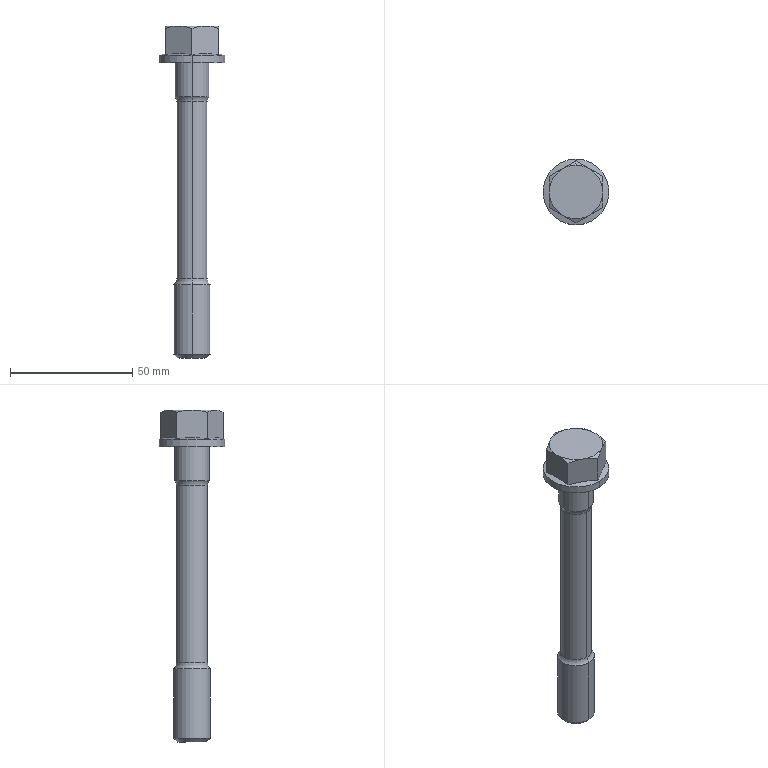Part | SolidWorks | features BaseBody 1 | 1 solid | 32 faces | box 27 x 27 x 136 mm | volume 23989 mm3 | cone 11 | plane 9 | cylinder 8 | torus 4 | commonest cylinder face diameters 12.7 x2 14 x2 15 x2 27 x2
STEP:
#1=CARTESIAN_POINT('',(-97.5,217.526,423.15));
#2=VERTEX_POINT('',#1);
#3=CARTESIAN_POINT('',(-92.,219.,423.15));
#4=VERTEX_POINT('',#3);
#5=CARTESIAN_POINT('',(-92.,208.,423.15));
#6=DIRECTION('',(0.,0.,-1.));
#7=DIRECTION('',(0.,-1.,0.));
#8=AXIS2_PLACEMENT_3D('',#5,#6,#7);
#9=CIRCLE('',#8,11.);
#10=EDGE_CURVE('',#2,#4,#9,.T.);
#11=ORIENTED_EDGE('',*,*,#10,.T.);
#12=CARTESIAN_POINT('',(-92.,220.702,422.168));
#13=VERTEX_POINT('',#12);
#14=CARTESIAN_POINT('',(-92.,216.604,424.533));
#15=DIRECTION('',(0.,0.866,-0.5));
#16=VECTOR('',#15,1000.);
#17=LINE('',#14,#16);
#18=EDGE_CURVE('',#4,#13,#17,.T.);
#19=ORIENTED_EDGE('',*,*,#18,.T.);
#20=CARTESIAN_POINT('',(-92.,220.702,422.168));
#21=CARTESIAN_POINT('',(-92.898,220.183,422.467));
#22=CARTESIAN_POINT('',(-93.804,219.66,422.714));
#23=CARTESIAN_POINT('',(-95.635,218.603,423.056));
#24=CARTESIAN_POINT('',(-96.561,218.068,423.15));
#25=CARTESIAN_POINT('',(-97.5,217.526,423.15));
#26=B_SPLINE_CURVE_WITH_KNOTS('',3,(#20,#21,#22,#23,#24,#25),.UNSPECIFIED.,.F.,.F.,(4,2,4),(0.,0.003213,0.006426),.UNSPECIFIED.);
#27=EDGE_CURVE('',#13,#2,#26,.T.);
#28=ORIENTED_EDGE('',*,*,#27,.T.);
#29=EDGE_LOOP('',(#11,#19,#28));
#30=FACE_OUTER_BOUND('',#29,.T.);
#31=CARTESIAN_POINT('',(-92.,208.,424.533));
#32=DIRECTION('',(0.,0.,-1.));
#33=DIRECTION('',(0.,1.,0.));
#34=AXIS2_PLACEMENT_3D('',#31,#32,#33);
#35=CONICAL_SURFACE('',#34,8.604,1.047);
#36=ADVANCED_FACE('',(#30),#35,.T.);
#37=CARTESIAN_POINT('',(-92.,221.5,411.15));
#38=VERTEX_POINT('',#37);
#39=CARTESIAN_POINT('',(-92.,194.5,411.15));
#40=VERTEX_POINT('',#39);
#41=CARTESIAN_POINT('',(-92.,208.,411.15));
#42=DIRECTION('',(0.,0.,-1.));
#43=DIRECTION('',(0.,1.,0.));
#44=AXIS2_PLACEMENT_3D('',#41,#42,#43);
#45=CIRCLE('',#44,13.5);
#46=EDGE_CURVE('',#38,#40,#45,.T.);
#47=ORIENTED_EDGE('',*,*,#46,.T.);
#48=CARTESIAN_POINT('',(-92.,194.5,408.15));
#49=VERTEX_POINT('',#48);
#50=CARTESIAN_POINT('',(-92.,194.5,414.767));
#51=DIRECTION('',(0.,0.,-1.));
#52=VECTOR('',#51,1000.);
#53=LINE('',#50,#52);
#54=EDGE_CURVE('',#40,#49,#53,.T.);
#55=ORIENTED_EDGE('',*,*,#54,.T.);
#56=CARTESIAN_POINT('',(-92.,221.5,408.15));
#57=VERTEX_POINT('',#56);
#58=CARTESIAN_POINT('',(-92.,208.,408.15));
#59=DIRECTION('',(0.,0.,-1.));
#60=DIRECTION('',(0.,1.,0.));
#61=AXIS2_PLACEMENT_3D('',#58,#59,#60);
#62=CIRCLE('',#61,13.5);
#63=EDGE_CURVE('',#57,#49,#62,.T.);
#64=ORIENTED_EDGE('',*,*,#63,.F.);
#65=CARTESIAN_POINT('',(-92.,221.5,414.767));
#66=DIRECTION('',(0.,0.,-1.));
#67=VECTOR('',#66,1000.);
#68=LINE('',#65,#67);
#69=EDGE_CURVE('',#38,#57,#68,.T.);
#70=ORIENTED_EDGE('',*,*,#69,.F.);
#71=EDGE_LOOP('',(#47,#55,#64,#70));
#72=FACE_OUTER_BOUND('',#71,.T.);
#73=CARTESIAN_POINT('',(-92.,208.,414.767));
#74=DIRECTION('',(0.,0.,-1.));
#75=DIRECTION('',(0.,1.,0.));
#76=AXIS2_PLACEMENT_3D('',#73,#74,#75);
#77=CYLINDRICAL_SURFACE('',#76,13.5);
#78=ADVANCED_FACE('',(#72),#77,.T.);
#79=CARTESIAN_POINT('',(-81.,201.649,411.364));
#80=VERTEX_POINT('',#79);
#81=CARTESIAN_POINT('',(-92.,195.298,411.364));
#82=VERTEX_POINT('',#81);
#83=CARTESIAN_POINT('',(-81.,201.649,411.364));
#84=CARTESIAN_POINT('',(-81.917,201.12,411.506));
#85=CARTESIAN_POINT('',(-82.833,200.591,411.621));
#86=CARTESIAN_POINT('',(-84.667,199.532,411.778));
#87=CARTESIAN_POINT('',(-86.5,198.474,411.862));
#88=CARTESIAN_POINT('',(-88.333,197.415,411.778));
#89=CARTESIAN_POINT('',(-90.167,196.357,411.621));
#90=CARTESIAN_POINT('',(-91.083,195.828,411.506));
#91=CARTESIAN_POINT('',(-92.,195.298,411.364));
#92=B_SPLINE_CURVE_WITH_KNOTS('',3,(#83,#84,#85,#86,#87,#88,#89,#90,#91),.UNSPECIFIED.,.F.,.F.,(4,2,1,2,4),(0.,0.003175,0.006351,0.009526,0.0127),.UNSPECIFIED.);
#93=EDGE_CURVE('',#80,#82,#92,.T.);
#94=ORIENTED_EDGE('',*,*,#93,.T.);
#95=CARTESIAN_POINT('',(-92.,194.5,411.15));
#96=DIRECTION('',(0.,-0.9659,-0.2588));
#97=VECTOR('',#96,1000.);
#98=LINE('',#95,#97);
#99=EDGE_CURVE('',#82,#40,#98,.T.);
#100=ORIENTED_EDGE('',*,*,#99,.T.);
#101=ORIENTED_EDGE('',*,*,#46,.F.);
#102=CARTESIAN_POINT('',(-92.,220.702,411.364));
#103=VERTEX_POINT('',#102);
#104=CARTESIAN_POINT('',(-92.,221.5,411.15));
#105=DIRECTION('',(0.,0.9659,-0.2588));
#106=VECTOR('',#105,1000.);
#107=LINE('',#104,#106);
#108=EDGE_CURVE('',#103,#38,#107,.T.);
#109=ORIENTED_EDGE('',*,*,#108,.F.);
#110=CARTESIAN_POINT('',(-81.,214.351,411.364));
#111=VERTEX_POINT('',#110);
#112=CARTESIAN_POINT('',(-92.,220.702,411.364));
#113=CARTESIAN_POINT('',(-91.083,220.172,411.506));
#114=CARTESIAN_POINT('',(-90.167,219.643,411.621));
#115=CARTESIAN_POINT('',(-88.333,218.585,411.778));
#116=CARTESIAN_POINT('',(-86.5,217.526,411.862));
#117=CARTESIAN_POINT('',(-84.667,216.468,411.778));
#118=CARTESIAN_POINT('',(-82.833,215.409,411.621));
#119=CARTESIAN_POINT('',(-81.917,214.88,411.506));
#120=CARTESIAN_POINT('',(-81.,214.351,411.364));
#121=B_SPLINE_CURVE_WITH_KNOTS('',3,(#112,#113,#114,#115,#116,#117,#118,#119,#120),.UNSPECIFIED.,.F.,.F.,(4,2,1,2,4),(0.,0.003175,0.006351,0.009526,0.0127),.UNSPECIFIED.);
#122=EDGE_CURVE('',#103,#111,#121,.T.);
#123=ORIENTED_EDGE('',*,*,#122,.T.);
#124=CARTESIAN_POINT('',(-81.,214.351,411.364));
#125=CARTESIAN_POINT('',(-81.,213.292,411.506));
#126=CARTESIAN_POINT('',(-81.,212.234,411.621));
#127=CARTESIAN_POINT('',(-81.,210.117,411.778));
#128=CARTESIAN_POINT('',(-81.,208.,411.862));
#129=CARTESIAN_POINT('',(-81.,205.883,411.778));
#130=CARTESIAN_POINT('',(-81.,203.766,411.621));
#131=CARTESIAN_POINT('',(-81.,202.708,411.506));
#132=CARTESIAN_POINT('',(-81.,201.649,411.364));
#133=B_SPLINE_CURVE_WITH_KNOTS('',3,(#124,#125,#126,#127,#128,#129,#130,#131,#132),.UNSPECIFIED.,.F.,.F.,(4,2,1,2,4),(0.,0.003175,0.006351,0.009526,0.0127),.UNSPECIFIED.);
#134=EDGE_CURVE('',#111,#80,#133,.T.);
#135=ORIENTED_EDGE('',*,*,#134,.T.);
#136=EDGE_LOOP('',(#94,#100,#101,#109,#123,#135));
#137=FACE_OUTER_BOUND('',#136,.T.);
#138=CARTESIAN_POINT('',(-92.,208.,411.15));
#139=DIRECTION('',(0.,0.,-1.));
#140=DIRECTION('',(0.,1.,0.));
#141=AXIS2_PLACEMENT_3D('',#138,#139,#140);
#142=CONICAL_SURFACE('',#141,13.5,1.309);
#143=ADVANCED_FACE('',(#137),#142,.T.);
#144=CARTESIAN_POINT('',(-92.,215.,408.15));
#145=VERTEX_POINT('',#144);
#146=CARTESIAN_POINT('',(-92.,201.,408.15));
#147=VERTEX_POINT('',#146);
#148=CARTESIAN_POINT('',(-92.,208.,408.15));
#149=DIRECTION('',(0.,0.,-1.));
#150=DIRECTION('',(0.,-1.,0.));
#151=AXIS2_PLACEMENT_3D('',#148,#149,#150);
#152=CIRCLE('',#151,7.);
#153=EDGE_CURVE('',#145,#147,#152,.T.);
#154=ORIENTED_EDGE('',*,*,#153,.T.);
#155=CARTESIAN_POINT('',(-92.,201.,394.15));
#156=VERTEX_POINT('',#155);
#157=CARTESIAN_POINT('',(-92.,201.,414.767));
#158=DIRECTION('',(0.,0.,-1.));
#159=VECTOR('',#158,1000.);
#160=LINE('',#157,#159);
#161=EDGE_CURVE('',#147,#156,#160,.T.);
#162=ORIENTED_EDGE('',*,*,#161,.T.);
#163=CARTESIAN_POINT('',(-92.,215.,394.15));
#164=VERTEX_POINT('',#163);
#165=CARTESIAN_POINT('',(-92.,208.,394.15));
#166=DIRECTION('',(0.,0.,-1.));
#167=DIRECTION('',(0.,1.,0.));
#168=AXIS2_PLACEMENT_3D('',#165,#166,#167);
#169=CIRCLE('',#168,7.);
#170=EDGE_CURVE('',#164,#156,#169,.T.);
#171=ORIENTED_EDGE('',*,*,#170,.F.);
#172=CARTESIAN_POINT('',(-92.,215.,414.767));
#173=DIRECTION('',(0.,0.,-1.));
#174=VECTOR('',#173,1000.);
#175=LINE('',#172,#174);
#176=EDGE_CURVE('',#145,#164,#175,.T.);
#177=ORIENTED_EDGE('',*,*,#176,.F.);
#178=EDGE_LOOP('',(#154,#162,#171,#177));
#179=FACE_OUTER_BOUND('',#178,.T.);
#180=CARTESIAN_POINT('',(-92.,208.,414.767));
#181=DIRECTION('',(0.,0.,-1.));
#182=DIRECTION('',(0.,1.,0.));
#183=AXIS2_PLACEMENT_3D('',#180,#181,#182);
#184=CYLINDRICAL_SURFACE('',#183,7.);
#185=ADVANCED_FACE('',(#179),#184,.T.);
#186=CARTESIAN_POINT('',(-92.,201.65,392.285));
#187=VERTEX_POINT('',#186);
#188=CARTESIAN_POINT('',(-92.,214.35,392.285));
#189=VERTEX_POINT('',#188);
#190=CARTESIAN_POINT('',(-92.,208.,392.285));
#191=DIRECTION('',(0.,0.,-1.));
#192=DIRECTION('',(0.,1.,0.));
#193=AXIS2_PLACEMENT_3D('',#190,#191,#192);
#194=CIRCLE('',#193,6.35);
#195=EDGE_CURVE('',#187,#189,#194,.T.);
#196=ORIENTED_EDGE('',*,*,#195,.F.);
#197=CARTESIAN_POINT('',(-92.,198.65,392.285));
#198=DIRECTION('',(1.,0.,0.));
#199=DIRECTION('',(0.,1.,0.));
#200=AXIS2_PLACEMENT_3D('',#197,#198,#199);
#201=CIRCLE('',#200,3.);
#202=EDGE_CURVE('',#187,#156,#201,.T.);
#203=ORIENTED_EDGE('',*,*,#202,.T.);
#204=CARTESIAN_POINT('',(-92.,208.,394.15));
#205=DIRECTION('',(0.,0.,-1.));
#206=DIRECTION('',(0.,1.,0.));
#207=AXIS2_PLACEMENT_3D('',#204,#205,#206);
#208=CIRCLE('',#207,7.);
#209=EDGE_CURVE('',#156,#164,#208,.T.);
#210=ORIENTED_EDGE('',*,*,#209,.T.);
#211=CARTESIAN_POINT('',(-92.,217.35,392.285));
#212=DIRECTION('',(-1.,0.,0.));
#213=DIRECTION('',(0.,0.,1.));
#214=AXIS2_PLACEMENT_3D('',#211,#212,#213);
#215=CIRCLE('',#214,3.);
#216=EDGE_CURVE('',#189,#164,#215,.T.);
#217=ORIENTED_EDGE('',*,*,#216,.F.);
#218=EDGE_LOOP('',(#196,#203,#210,#217));
#219=FACE_OUTER_BOUND('',#218,.T.);
#220=CARTESIAN_POINT('',(-92.,208.,392.285));
#221=DIRECTION('',(0.,0.,-1.));
#222=DIRECTION('',(0.,1.,0.));
#223=AXIS2_PLACEMENT_3D('',#220,#221,#222);
#224=TOROIDAL_SURFACE('',#223,9.35,3.);
#225=ADVANCED_FACE('',(#219),#224,.F.);
#226=CARTESIAN_POINT('',(-92.,208.,392.285));
#227=DIRECTION('',(0.,0.,-1.));
#228=DIRECTION('',(0.,1.,0.));
#229=AXIS2_PLACEMENT_3D('',#226,#227,#228);
#230=CIRCLE('',#229,6.35);
#231=EDGE_CURVE('',#189,#187,#230,.T.);
#232=ORIENTED_EDGE('',*,*,#231,.T.);
#233=CARTESIAN_POINT('',(-92.,201.65,319.512));
#234=VERTEX_POINT('',#233);
#235=CARTESIAN_POINT('',(-92.,201.65,414.767));
#236=DIRECTION('',(0.,0.,-1.));
#237=VECTOR('',#236,1000.);
#238=LINE('',#235,#237);
#239=EDGE_CURVE('',#187,#234,#238,.T.);
#240=ORIENTED_EDGE('',*,*,#239,.T.);
#241=CARTESIAN_POINT('',(-92.,214.35,319.512));
#242=VERTEX_POINT('',#241);
#243=CARTESIAN_POINT('',(-92.,208.,319.512));
#244=DIRECTION('',(0.,0.,-1.));
#245=DIRECTION('',(0.,1.,0.));
#246=AXIS2_PLACEMENT_3D('',#243,#244,#245);
#247=CIRCLE('',#246,6.35);
#248=EDGE_CURVE('',#242,#234,#247,.T.);
#249=ORIENTED_EDGE('',*,*,#248,.F.);
#250=CARTESIAN_POINT('',(-92.,214.35,414.767));
#251=DIRECTION('',(0.,0.,-1.));
#252=VECTOR('',#251,1000.);
#253=LINE('',#250,#252);
#254=EDGE_CURVE('',#189,#242,#253,.T.);
#255=ORIENTED_EDGE('',*,*,#254,.F.);
#256=EDGE_LOOP('',(#232,#240,#249,#255));
#257=FACE_OUTER_BOUND('',#256,.T.);
#258=CARTESIAN_POINT('',(-92.,208.,414.767));
#259=DIRECTION('',(0.,0.,-1.));
#260=DIRECTION('',(0.,1.,0.));
#261=AXIS2_PLACEMENT_3D('',#258,#259,#260);
#262=CYLINDRICAL_SURFACE('',#261,6.35);
#263=ADVANCED_FACE('',(#257),#262,.T.);
#264=CARTESIAN_POINT('',(-92.,200.5,317.15));
#265=VERTEX_POINT('',#264);
#266=CARTESIAN_POINT('',(-92.,215.5,317.15));
#267=VERTEX_POINT('',#266);
#268=CARTESIAN_POINT('',(-92.,208.,317.15));
#269=DIRECTION('',(0.,0.,-1.));
#270=DIRECTION('',(0.,1.,0.));
#271=AXIS2_PLACEMENT_3D('',#268,#269,#270);
#272=CIRCLE('',#271,7.5);
#273=EDGE_CURVE('',#265,#267,#272,.T.);
#274=ORIENTED_EDGE('',*,*,#273,.F.);
#275=CARTESIAN_POINT('',(-92.,198.65,319.512));
#276=DIRECTION('',(1.,0.,0.));
#277=DIRECTION('',(0.,1.,0.));
#278=AXIS2_PLACEMENT_3D('',#275,#276,#277);
#279=CIRCLE('',#278,3.);
#280=EDGE_CURVE('',#265,#234,#279,.T.);
#281=ORIENTED_EDGE('',*,*,#280,.T.);
#282=CARTESIAN_POINT('',(-92.,208.,319.512));
#283=DIRECTION('',(0.,0.,-1.));
#284=DIRECTION('',(0.,1.,0.));
#285=AXIS2_PLACEMENT_3D('',#282,#283,#284);
#286=CIRCLE('',#285,6.35);
#287=EDGE_CURVE('',#234,#242,#286,.T.);
#288=ORIENTED_EDGE('',*,*,#287,.T.);
#289=CARTESIAN_POINT('',(-92.,217.35,319.512));
#290=DIRECTION('',(-1.,0.,0.));
#291=DIRECTION('',(0.,0.,1.));
#292=AXIS2_PLACEMENT_3D('',#289,#290,#291);
#293=CIRCLE('',#292,3.);
#294=EDGE_CURVE('',#267,#242,#293,.T.);
#295=ORIENTED_EDGE('',*,*,#294,.F.);
#296=EDGE_LOOP('',(#274,#281,#288,#295));
#297=FACE_OUTER_BOUND('',#296,.T.);
#298=CARTESIAN_POINT('',(-92.,208.,319.512));
#299=DIRECTION('',(0.,0.,-1.));
#300=DIRECTION('',(0.,1.,0.));
#301=AXIS2_PLACEMENT_3D('',#298,#299,#300);
#302=TOROIDAL_SURFACE('',#301,9.35,3.);
#303=ADVANCED_FACE('',(#297),#302,.F.);
#304=CARTESIAN_POINT('',(-92.,208.,317.15));
#305=DIRECTION('',(0.,0.,-1.));
#306=DIRECTION('',(0.,1.,0.));
#307=AXIS2_PLACEMENT_3D('',#304,#305,#306);
#308=CIRCLE('',#307,7.5);
#309=EDGE_CURVE('',#267,#265,#308,.T.);
#310=ORIENTED_EDGE('',*,*,#309,.T.);
#311=CARTESIAN_POINT('',(-92.,200.5,288.65));
#312=VERTEX_POINT('',#311);
#313=CARTESIAN_POINT('',(-92.,200.5,414.767));
#314=DIRECTION('',(0.,0.,-1.));
#315=VECTOR('',#314,1000.);
#316=LINE('',#313,#315);
#317=EDGE_CURVE('',#265,#312,#316,.T.);
#318=ORIENTED_EDGE('',*,*,#317,.T.);
#319=CARTESIAN_POINT('',(-92.,215.5,288.65));
#320=VERTEX_POINT('',#319);
#321=CARTESIAN_POINT('',(-92.,208.,288.65));
#322=DIRECTION('',(0.,0.,-1.));
#323=DIRECTION('',(0.,1.,0.));
#324=AXIS2_PLACEMENT_3D('',#321,#322,#323);
#325=CIRCLE('',#324,7.5);
#326=EDGE_CURVE('',#320,#312,#325,.T.);
#327=ORIENTED_EDGE('',*,*,#326,.F.);
#328=CARTESIAN_POINT('',(-92.,215.5,414.767));
#329=DIRECTION('',(0.,0.,-1.));
#330=VECTOR('',#329,1000.);
#331=LINE('',#328,#330);
#332=EDGE_CURVE('',#267,#320,#331,.T.);
#333=ORIENTED_EDGE('',*,*,#332,.F.);
#334=EDGE_LOOP('',(#310,#318,#327,#333));
#335=FACE_OUTER_BOUND('',#334,.T.);
#336=CARTESIAN_POINT('',(-92.,208.,414.767));
#337=DIRECTION('',(0.,0.,-1.));
#338=DIRECTION('',(0.,1.,0.));
#339=AXIS2_PLACEMENT_3D('',#336,#337,#338);
#340=CYLINDRICAL_SURFACE('',#339,7.5);
#341=ADVANCED_FACE('',(#335),#340,.T.);
#342=CARTESIAN_POINT('',(-92.,214.,287.15));
#343=VERTEX_POINT('',#342);
#344=CARTESIAN_POINT('',(-92.,202.,287.15));
#345=VERTEX_POINT('',#344);
#346=CARTESIAN_POINT('',(-92.,208.,287.15));
#347=DIRECTION('',(0.,0.,-1.));
#348=DIRECTION('',(0.,1.,0.));
#349=AXIS2_PLACEMENT_3D('',#346,#347,#348);
#350=CIRCLE('',#349,6.);
#351=EDGE_CURVE('',#343,#345,#350,.T.);
#352=ORIENTED_EDGE('',*,*,#351,.F.);
#353=CARTESIAN_POINT('',(-92.,214.,287.15));
#354=DIRECTION('',(0.,0.7071,0.7071));
#355=VECTOR('',#354,1000.);
#356=LINE('',#353,#355);
#357=EDGE_CURVE('',#343,#320,#356,.T.);
#358=ORIENTED_EDGE('',*,*,#357,.T.);
#359=ORIENTED_EDGE('',*,*,#326,.T.);
#360=CARTESIAN_POINT('',(-92.,202.,287.15));
#361=DIRECTION('',(0.,-0.7071,0.7071));
#362=VECTOR('',#361,1000.);
#363=LINE('',#360,#362);
#364=EDGE_CURVE('',#345,#312,#363,.T.);
#365=ORIENTED_EDGE('',*,*,#364,.F.);
#366=EDGE_LOOP('',(#352,#358,#359,#365));
#367=FACE_OUTER_BOUND('',#366,.T.);
#368=CARTESIAN_POINT('',(-92.,208.,287.15));
#369=DIRECTION('',(0.,0.,1.));
#370=DIRECTION('',(0.,-1.,0.));
#371=AXIS2_PLACEMENT_3D('',#368,#369,#370);
#372=CONICAL_SURFACE('',#371,6.,0.7854);
#373=ADVANCED_FACE('',(#367),#372,.T.);
#374=CARTESIAN_POINT('',(-92.,208.,287.15));
#375=DIRECTION('',(0.,0.,-1.));
#376=DIRECTION('',(0.,1.,0.));
#377=AXIS2_PLACEMENT_3D('',#374,#375,#376);
#378=CIRCLE('',#377,6.);
#379=EDGE_CURVE('',#345,#343,#378,.T.);
#380=ORIENTED_EDGE('',*,*,#379,.T.);
#381=ORIENTED_EDGE('',*,*,#351,.T.);
#382=EDGE_LOOP('',(#380,#381));
#383=FACE_OUTER_BOUND('',#382,.T.);
#384=CARTESIAN_POINT('',(-92.,208.,287.15));
#385=DIRECTION('',(0.,0.,-1.));
#386=DIRECTION('',(0.,-1.,0.));
#387=AXIS2_PLACEMENT_3D('',#384,#385,#386);
#388=PLANE('',#387);
#389=ADVANCED_FACE('',(#383),#388,.T.);
#390=ORIENTED_EDGE('',*,*,#357,.F.);
#391=ORIENTED_EDGE('',*,*,#379,.F.);
#392=ORIENTED_EDGE('',*,*,#364,.T.);
#393=CARTESIAN_POINT('',(-92.,208.,288.65));
#394=DIRECTION('',(0.,0.,-1.));
#395=DIRECTION('',(0.,1.,0.));
#396=AXIS2_PLACEMENT_3D('',#393,#394,#395);
#397=CIRCLE('',#396,7.5);
#398=EDGE_CURVE('',#312,#320,#397,.T.);
#399=ORIENTED_EDGE('',*,*,#398,.T.);
#400=EDGE_LOOP('',(#390,#391,#392,#399));
#401=FACE_OUTER_BOUND('',#400,.T.);
#402=CARTESIAN_POINT('',(-92.,208.,287.15));
#403=DIRECTION('',(0.,0.,1.));
#404=DIRECTION('',(0.,-1.,0.));
#405=AXIS2_PLACEMENT_3D('',#402,#403,#404);
#406=CONICAL_SURFACE('',#405,6.,0.7854);
#407=ADVANCED_FACE('',(#401),#406,.T.);
#408=ORIENTED_EDGE('',*,*,#317,.F.);
#409=ORIENTED_EDGE('',*,*,#273,.T.);
#410=ORIENTED_EDGE('',*,*,#332,.T.);
#411=ORIENTED_EDGE('',*,*,#398,.F.);
#412=EDGE_LOOP('',(#408,#409,#410,#411));
#413=FACE_OUTER_BOUND('',#412,.T.);
#414=CARTESIAN_POINT('',(-92.,208.,414.767));
#415=DIRECTION('',(0.,0.,-1.));
#416=DIRECTION('',(0.,1.,0.));
#417=AXIS2_PLACEMENT_3D('',#414,#415,#416);
#418=CYLINDRICAL_SURFACE('',#417,7.5);
#419=ADVANCED_FACE('',(#413),#418,.T.);
#420=ORIENTED_EDGE('',*,*,#280,.F.);
#421=ORIENTED_EDGE('',*,*,#309,.F.);
#422=ORIENTED_EDGE('',*,*,#294,.T.);
#423=ORIENTED_EDGE('',*,*,#248,.T.);
#424=EDGE_LOOP('',(#420,#421,#422,#423));
#425=FACE_OUTER_BOUND('',#424,.T.);
#426=CARTESIAN_POINT('',(-92.,208.,319.512));
#427=DIRECTION('',(0.,0.,-1.));
#428=DIRECTION('',(0.,1.,0.));
#429=AXIS2_PLACEMENT_3D('',#426,#427,#428);
#430=TOROIDAL_SURFACE('',#429,9.35,3.);
#431=ADVANCED_FACE('',(#425),#430,.F.);
#432=ORIENTED_EDGE('',*,*,#239,.F.);
#433=ORIENTED_EDGE('',*,*,#195,.T.);
#434=ORIENTED_EDGE('',*,*,#254,.T.);
#435=ORIENTED_EDGE('',*,*,#287,.F.);
#436=EDGE_LOOP('',(#432,#433,#434,#435));
#437=FACE_OUTER_BOUND('',#436,.T.);
#438=CARTESIAN_POINT('',(-92.,208.,414.767));
#439=DIRECTION('',(0.,0.,-1.));
#440=DIRECTION('',(0.,1.,0.));
#441=AXIS2_PLACEMENT_3D('',#438,#439,#440);
#442=CYLINDRICAL_SURFACE('',#441,6.35);
#443=ADVANCED_FACE('',(#437),#442,.T.);
#444=ORIENTED_EDGE('',*,*,#202,.F.);
#445=ORIENTED_EDGE('',*,*,#231,.F.);
#446=ORIENTED_EDGE('',*,*,#216,.T.);
#447=ORIENTED_EDGE('',*,*,#170,.T.);
#448=EDGE_LOOP('',(#444,#445,#446,#447));
#449=FACE_OUTER_BOUND('',#448,.T.);
#450=CARTESIAN_POINT('',(-92.,208.,392.285));
#451=DIRECTION('',(0.,0.,-1.));
#452=DIRECTION('',(0.,1.,0.));
#453=AXIS2_PLACEMENT_3D('',#450,#451,#452);
#454=TOROIDAL_SURFACE('',#453,9.35,3.);
#455=ADVANCED_FACE('',(#449),#454,.F.);
#456=ORIENTED_EDGE('',*,*,#161,.F.);
#457=CARTESIAN_POINT('',(-92.,208.,408.15));
#458=DIRECTION('',(0.,0.,-1.));
#459=DIRECTION('',(0.,-1.,0.));
#460=AXIS2_PLACEMENT_3D('',#457,#458,#459);
#461=CIRCLE('',#460,7.);
#462=EDGE_CURVE('',#147,#145,#461,.T.);
#463=ORIENTED_EDGE('',*,*,#462,.T.);
#464=ORIENTED_EDGE('',*,*,#176,.T.);
#465=ORIENTED_EDGE('',*,*,#209,.F.);
#466=EDGE_LOOP('',(#456,#463,#464,#465));
#467=FACE_OUTER_BOUND('',#466,.T.);
#468=CARTESIAN_POINT('',(-92.,208.,414.767));
#469=DIRECTION('',(0.,0.,-1.));
#470=DIRECTION('',(0.,1.,0.));
#471=AXIS2_PLACEMENT_3D('',#468,#469,#470);
#472=CYLINDRICAL_SURFACE('',#471,7.);
#473=ADVANCED_FACE('',(#467),#472,.T.);
#474=ORIENTED_EDGE('',*,*,#63,.T.);
#475=CARTESIAN_POINT('',(-92.,208.,408.15));
#476=DIRECTION('',(0.,0.,-1.));
#477=DIRECTION('',(0.,1.,0.));
#478=AXIS2_PLACEMENT_3D('',#475,#476,#477);
#479=CIRCLE('',#478,13.5);
#480=EDGE_CURVE('',#49,#57,#479,.T.);
#481=ORIENTED_EDGE('',*,*,#480,.T.);
#482=EDGE_LOOP('',(#474,#481));
#483=FACE_OUTER_BOUND('',#482,.T.);
#484=ORIENTED_EDGE('',*,*,#153,.F.);
#485=ORIENTED_EDGE('',*,*,#462,.F.);
#486=EDGE_LOOP('',(#484,#485));
#487=FACE_BOUND('',#486,.T.);
#488=CARTESIAN_POINT('',(-103.,227.053,408.15));
#489=DIRECTION('',(0.,0.,1.));
#490=DIRECTION('',(1.,0.,0.));
#491=AXIS2_PLACEMENT_3D('',#488,#489,#490);
#492=PLANE('',#491);
#493=ADVANCED_FACE('',(#483,#487),#492,.F.);
#494=ORIENTED_EDGE('',*,*,#99,.F.);
#495=CARTESIAN_POINT('',(-103.,201.649,411.364));
#496=VERTEX_POINT('',#495);
#497=CARTESIAN_POINT('',(-92.,195.298,411.364));
#498=CARTESIAN_POINT('',(-92.917,195.828,411.506));
#499=CARTESIAN_POINT('',(-93.833,196.357,411.621));
#500=CARTESIAN_POINT('',(-95.667,197.415,411.778));
#501=CARTESIAN_POINT('',(-97.5,198.474,411.862));
#502=CARTESIAN_POINT('',(-99.333,199.532,411.778));
#503=CARTESIAN_POINT('',(-101.167,200.591,411.621));
#504=CARTESIAN_POINT('',(-102.083,201.12,411.506));
#505=CARTESIAN_POINT('',(-103.,201.649,411.364));
#506=B_SPLINE_CURVE_WITH_KNOTS('',3,(#497,#498,#499,#500,#501,#502,#503,#504,#505),.UNSPECIFIED.,.F.,.F.,(4,2,1,2,4),(0.,0.003175,0.006351,0.009526,0.0127),.UNSPECIFIED.);
#507=EDGE_CURVE('',#82,#496,#506,.T.);
#508=ORIENTED_EDGE('',*,*,#507,.T.);
#509=CARTESIAN_POINT('',(-103.,214.351,411.364));
#510=VERTEX_POINT('',#509);
#511=CARTESIAN_POINT('',(-103.,201.649,411.364));
#512=CARTESIAN_POINT('',(-103.,202.708,411.506));
#513=CARTESIAN_POINT('',(-103.,203.766,411.621));
#514=CARTESIAN_POINT('',(-103.,205.883,411.778));
#515=CARTESIAN_POINT('',(-103.,208.,411.862));
#516=CARTESIAN_POINT('',(-103.,210.117,411.778));
#517=CARTESIAN_POINT('',(-103.,212.234,411.621));
#518=CARTESIAN_POINT('',(-103.,213.292,411.506));
#519=CARTESIAN_POINT('',(-103.,214.351,411.364));
#520=B_SPLINE_CURVE_WITH_KNOTS('',3,(#511,#512,#513,#514,#515,#516,#517,#518,#519),.UNSPECIFIED.,.F.,.F.,(4,2,1,2,4),(0.,0.003175,0.006351,0.009526,0.0127),.UNSPECIFIED.);
#521=EDGE_CURVE('',#496,#510,#520,.T.);
#522=ORIENTED_EDGE('',*,*,#521,.T.);
#523=CARTESIAN_POINT('',(-103.,214.351,411.364));
#524=CARTESIAN_POINT('',(-102.083,214.88,411.506));
#525=CARTESIAN_POINT('',(-101.167,215.409,411.621));
#526=CARTESIAN_POINT('',(-99.333,216.468,411.778));
#527=CARTESIAN_POINT('',(-97.5,217.526,411.862));
#528=CARTESIAN_POINT('',(-95.667,218.585,411.778));
#529=CARTESIAN_POINT('',(-93.833,219.643,411.621));
#530=CARTESIAN_POINT('',(-92.917,220.172,411.506));
#531=CARTESIAN_POINT('',(-92.,220.702,411.364));
#532=B_SPLINE_CURVE_WITH_KNOTS('',3,(#523,#524,#525,#526,#527,#528,#529,#530,#531),.UNSPECIFIED.,.F.,.F.,(4,2,1,2,4),(0.,0.003175,0.006351,0.009526,0.0127),.UNSPECIFIED.);
#533=EDGE_CURVE('',#510,#103,#532,.T.);
#534=ORIENTED_EDGE('',*,*,#533,.T.);
#535=ORIENTED_EDGE('',*,*,#108,.T.);
#536=CARTESIAN_POINT('',(-92.,208.,411.15));
#537=DIRECTION('',(0.,0.,-1.));
#538=DIRECTION('',(0.,1.,0.));
#539=AXIS2_PLACEMENT_3D('',#536,#537,#538);
#540=CIRCLE('',#539,13.5);
#541=EDGE_CURVE('',#40,#38,#540,.T.);
#542=ORIENTED_EDGE('',*,*,#541,.F.);
#543=EDGE_LOOP('',(#494,#508,#522,#534,#535,#542));
#544=FACE_OUTER_BOUND('',#543,.T.);
#545=CARTESIAN_POINT('',(-92.,208.,411.15));
#546=DIRECTION('',(0.,0.,-1.));
#547=DIRECTION('',(0.,1.,0.));
#548=AXIS2_PLACEMENT_3D('',#545,#546,#547);
#549=CONICAL_SURFACE('',#548,13.5,1.309);
#550=ADVANCED_FACE('',(#544),#549,.T.);
#551=ORIENTED_EDGE('',*,*,#54,.F.);
#552=ORIENTED_EDGE('',*,*,#541,.T.);
#553=ORIENTED_EDGE('',*,*,#69,.T.);
#554=ORIENTED_EDGE('',*,*,#480,.F.);
#555=EDGE_LOOP('',(#551,#552,#553,#554));
#556=FACE_OUTER_BOUND('',#555,.T.);
#557=CARTESIAN_POINT('',(-92.,208.,414.767));
#558=DIRECTION('',(0.,0.,-1.));
#559=DIRECTION('',(0.,1.,0.));
#560=AXIS2_PLACEMENT_3D('',#557,#558,#559);
#561=CYLINDRICAL_SURFACE('',#560,13.5);
#562=ADVANCED_FACE('',(#556),#561,.T.);
#563=CARTESIAN_POINT('',(-97.5,198.474,423.15));
#564=VERTEX_POINT('',#563);
#565=CARTESIAN_POINT('',(-103.,208.,423.15));
#566=VERTEX_POINT('',#565);
#567=CARTESIAN_POINT('',(-92.,208.,423.15));
#568=DIRECTION('',(0.,0.,-1.));
#569=DIRECTION('',(0.,-1.,0.));
#570=AXIS2_PLACEMENT_3D('',#567,#568,#569);
#571=CIRCLE('',#570,11.);
#572=EDGE_CURVE('',#564,#566,#571,.T.);
#573=ORIENTED_EDGE('',*,*,#572,.F.);
#574=CARTESIAN_POINT('',(-86.5,198.474,423.15));
#575=VERTEX_POINT('',#574);
#576=CARTESIAN_POINT('',(-92.,208.,423.15));
#577=DIRECTION('',(0.,0.,-1.));
#578=DIRECTION('',(0.,-1.,0.));
#579=AXIS2_PLACEMENT_3D('',#576,#577,#578);
#580=CIRCLE('',#579,11.);
#581=EDGE_CURVE('',#575,#564,#580,.T.);
#582=ORIENTED_EDGE('',*,*,#581,.F.);
#583=CARTESIAN_POINT('',(-81.,208.,423.15));
#584=VERTEX_POINT('',#583);
#585=CARTESIAN_POINT('',(-92.,208.,423.15));
#586=DIRECTION('',(0.,0.,-1.));
#587=DIRECTION('',(0.,-1.,0.));
#588=AXIS2_PLACEMENT_3D('',#585,#586,#587);
#589=CIRCLE('',#588,11.);
#590=EDGE_CURVE('',#584,#575,#589,.T.);
#591=ORIENTED_EDGE('',*,*,#590,.F.);
#592=CARTESIAN_POINT('',(-86.5,217.526,423.15));
#593=VERTEX_POINT('',#592);
#594=CARTESIAN_POINT('',(-92.,208.,423.15));
#595=DIRECTION('',(0.,0.,-1.));
#596=DIRECTION('',(0.,-1.,0.));
#597=AXIS2_PLACEMENT_3D('',#594,#595,#596);
#598=CIRCLE('',#597,11.);
#599=EDGE_CURVE('',#593,#584,#598,.T.);
#600=ORIENTED_EDGE('',*,*,#599,.F.);
#601=CARTESIAN_POINT('',(-92.,208.,423.15));
#602=DIRECTION('',(0.,0.,-1.));
#603=DIRECTION('',(0.,-1.,0.));
#604=AXIS2_PLACEMENT_3D('',#601,#602,#603);
#605=CIRCLE('',#604,11.);
#606=EDGE_CURVE('',#4,#593,#605,.T.);
#607=ORIENTED_EDGE('',*,*,#606,.F.);
#608=ORIENTED_EDGE('',*,*,#10,.F.);
#609=CARTESIAN_POINT('',(-92.,208.,423.15));
#610=DIRECTION('',(0.,0.,-1.));
#611=DIRECTION('',(0.,-1.,0.));
#612=AXIS2_PLACEMENT_3D('',#609,#610,#611);
#613=CIRCLE('',#612,11.);
#614=EDGE_CURVE('',#566,#2,#613,.T.);
#615=ORIENTED_EDGE('',*,*,#614,.F.);
#616=EDGE_LOOP('',(#573,#582,#591,#600,#607,#608,#615));
#617=FACE_OUTER_BOUND('',#616,.T.);
#618=CARTESIAN_POINT('',(-103.,227.053,423.15));
#619=DIRECTION('',(0.,0.,1.));
#620=DIRECTION('',(1.,0.,0.));
#621=AXIS2_PLACEMENT_3D('',#618,#619,#620);
#622=PLANE('',#621);
#623=ADVANCED_FACE('',(#617),#622,.T.);
#624=CARTESIAN_POINT('',(-103.,201.649,422.168));
#625=VERTEX_POINT('',#624);
#626=CARTESIAN_POINT('',(-103.,201.649,422.168));
#627=CARTESIAN_POINT('',(-102.102,201.13,422.467));
#628=CARTESIAN_POINT('',(-101.196,200.608,422.714));
#629=CARTESIAN_POINT('',(-99.365,199.55,423.056));
#630=CARTESIAN_POINT('',(-98.439,199.016,423.15));
#631=CARTESIAN_POINT('',(-97.5,198.474,423.15));
#632=B_SPLINE_CURVE_WITH_KNOTS('',3,(#626,#627,#628,#629,#630,#631),.UNSPECIFIED.,.F.,.F.,(4,2,4),(0.,0.003213,0.006426),.UNSPECIFIED.);
#633=EDGE_CURVE('',#625,#564,#632,.T.);
#634=ORIENTED_EDGE('',*,*,#633,.T.);
#635=ORIENTED_EDGE('',*,*,#572,.T.);
#636=CARTESIAN_POINT('',(-103.,208.,423.15));
#637=CARTESIAN_POINT('',(-103.,206.916,423.15));
#638=CARTESIAN_POINT('',(-103.,205.847,423.056));
#639=CARTESIAN_POINT('',(-103.,203.732,422.714));
#640=CARTESIAN_POINT('',(-103.,202.687,422.467));
#641=CARTESIAN_POINT('',(-103.,201.649,422.168));
#642=B_SPLINE_CURVE_WITH_KNOTS('',3,(#636,#637,#638,#639,#640,#641),.UNSPECIFIED.,.F.,.F.,(4,2,4),(0.,0.003213,0.006426),.UNSPECIFIED.);
#643=EDGE_CURVE('',#566,#625,#642,.T.);
#644=ORIENTED_EDGE('',*,*,#643,.T.);
#645=EDGE_LOOP('',(#634,#635,#644));
#646=FACE_OUTER_BOUND('',#645,.T.);
#647=CARTESIAN_POINT('',(-92.,208.,424.533));
#648=DIRECTION('',(0.,0.,-1.));
#649=DIRECTION('',(0.,1.,0.));
#650=AXIS2_PLACEMENT_3D('',#647,#648,#649);
#651=CONICAL_SURFACE('',#650,8.604,1.047);
#652=ADVANCED_FACE('',(#646),#651,.T.);
#653=CARTESIAN_POINT('',(-103.,214.351,422.168));
#654=VERTEX_POINT('',#653);
#655=CARTESIAN_POINT('',(-103.,214.351,422.168));
#656=CARTESIAN_POINT('',(-103.,213.313,422.467));
#657=CARTESIAN_POINT('',(-103.,212.268,422.714));
#658=CARTESIAN_POINT('',(-103.,210.153,423.056));
#659=CARTESIAN_POINT('',(-103.,209.084,423.15));
#660=CARTESIAN_POINT('',(-103.,208.,423.15));
#661=B_SPLINE_CURVE_WITH_KNOTS('',3,(#655,#656,#657,#658,#659,#660),.UNSPECIFIED.,.F.,.F.,(4,2,4),(0.,0.003213,0.006426),.UNSPECIFIED.);
#662=EDGE_CURVE('',#654,#566,#661,.T.);
#663=ORIENTED_EDGE('',*,*,#662,.T.);
#664=ORIENTED_EDGE('',*,*,#614,.T.);
#665=CARTESIAN_POINT('',(-97.5,217.526,423.15));
#666=CARTESIAN_POINT('',(-98.439,216.984,423.15));
#667=CARTESIAN_POINT('',(-99.365,216.45,423.056));
#668=CARTESIAN_POINT('',(-101.196,215.392,422.714));
#669=CARTESIAN_POINT('',(-102.102,214.87,422.467));
#670=CARTESIAN_POINT('',(-103.,214.351,422.168));
#671=B_SPLINE_CURVE_WITH_KNOTS('',3,(#665,#666,#667,#668,#669,#670),.UNSPECIFIED.,.F.,.F.,(4,2,4),(0.,0.003213,0.006426),.UNSPECIFIED.);
#672=EDGE_CURVE('',#2,#654,#671,.T.);
#673=ORIENTED_EDGE('',*,*,#672,.T.);
#674=EDGE_LOOP('',(#663,#664,#673));
#675=FACE_OUTER_BOUND('',#674,.T.);
#676=CARTESIAN_POINT('',(-92.,208.,424.533));
#677=DIRECTION('',(0.,0.,-1.));
#678=DIRECTION('',(0.,1.,0.));
#679=AXIS2_PLACEMENT_3D('',#676,#677,#678);
#680=CONICAL_SURFACE('',#679,8.604,1.047);
#681=ADVANCED_FACE('',(#675),#680,.T.);
#682=ORIENTED_EDGE('',*,*,#18,.F.);
#683=ORIENTED_EDGE('',*,*,#606,.T.);
#684=CARTESIAN_POINT('',(-86.5,217.526,423.15));
#685=CARTESIAN_POINT('',(-87.439,218.068,423.15));
#686=CARTESIAN_POINT('',(-88.365,218.603,423.056));
#687=CARTESIAN_POINT('',(-90.196,219.66,422.714));
#688=CARTESIAN_POINT('',(-91.102,220.183,422.467));
#689=CARTESIAN_POINT('',(-92.,220.702,422.168));
#690=B_SPLINE_CURVE_WITH_KNOTS('',3,(#684,#685,#686,#687,#688,#689),.UNSPECIFIED.,.F.,.F.,(4,2,4),(0.,0.003213,0.006426),.UNSPECIFIED.);
#691=EDGE_CURVE('',#593,#13,#690,.T.);
#692=ORIENTED_EDGE('',*,*,#691,.T.);
#693=EDGE_LOOP('',(#682,#683,#692));
#694=FACE_OUTER_BOUND('',#693,.T.);
#695=CARTESIAN_POINT('',(-92.,208.,424.533));
#696=DIRECTION('',(0.,0.,-1.));
#697=DIRECTION('',(0.,1.,0.));
#698=AXIS2_PLACEMENT_3D('',#695,#696,#697);
#699=CONICAL_SURFACE('',#698,8.604,1.047);
#700=ADVANCED_FACE('',(#694),#699,.T.);
#701=CARTESIAN_POINT('',(-81.,214.351,422.168));
#702=VERTEX_POINT('',#701);
#703=CARTESIAN_POINT('',(-81.,214.351,422.168));
#704=CARTESIAN_POINT('',(-81.898,214.87,422.467));
#705=CARTESIAN_POINT('',(-82.804,215.392,422.714));
#706=CARTESIAN_POINT('',(-84.635,216.45,423.056));
#707=CARTESIAN_POINT('',(-85.561,216.984,423.15));
#708=CARTESIAN_POINT('',(-86.5,217.526,423.15));
#709=B_SPLINE_CURVE_WITH_KNOTS('',3,(#703,#704,#705,#706,#707,#708),.UNSPECIFIED.,.F.,.F.,(4,2,4),(0.,0.003213,0.006426),.UNSPECIFIED.);
#710=EDGE_CURVE('',#702,#593,#709,.T.);
#711=ORIENTED_EDGE('',*,*,#710,.T.);
#712=ORIENTED_EDGE('',*,*,#599,.T.);
#713=CARTESIAN_POINT('',(-81.,208.,423.15));
#714=CARTESIAN_POINT('',(-81.,209.084,423.15));
#715=CARTESIAN_POINT('',(-81.,210.153,423.056));
#716=CARTESIAN_POINT('',(-81.,212.268,422.714));
#717=CARTESIAN_POINT('',(-81.,213.313,422.467));
#718=CARTESIAN_POINT('',(-81.,214.351,422.168));
#719=B_SPLINE_CURVE_WITH_KNOTS('',3,(#713,#714,#715,#716,#717,#718),.UNSPECIFIED.,.F.,.F.,(4,2,4),(0.,0.003213,0.006426),.UNSPECIFIED.);
#720=EDGE_CURVE('',#584,#702,#719,.T.);
#721=ORIENTED_EDGE('',*,*,#720,.T.);
#722=EDGE_LOOP('',(#711,#712,#721));
#723=FACE_OUTER_BOUND('',#722,.T.);
#724=CARTESIAN_POINT('',(-92.,208.,424.533));
#725=DIRECTION('',(0.,0.,-1.));
#726=DIRECTION('',(0.,1.,0.));
#727=AXIS2_PLACEMENT_3D('',#724,#725,#726);
#728=CONICAL_SURFACE('',#727,8.604,1.047);
#729=ADVANCED_FACE('',(#723),#728,.T.);
#730=CARTESIAN_POINT('',(-81.,201.649,422.168));
#731=VERTEX_POINT('',#730);
#732=CARTESIAN_POINT('',(-81.,201.649,422.168));
#733=CARTESIAN_POINT('',(-81.,202.687,422.467));
#734=CARTESIAN_POINT('',(-81.,203.732,422.714));
#735=CARTESIAN_POINT('',(-81.,205.847,423.056));
#736=CARTESIAN_POINT('',(-81.,206.916,423.15));
#737=CARTESIAN_POINT('',(-81.,208.,423.15));
#738=B_SPLINE_CURVE_WITH_KNOTS('',3,(#732,#733,#734,#735,#736,#737),.UNSPECIFIED.,.F.,.F.,(4,2,4),(0.,0.003213,0.006426),.UNSPECIFIED.);
#739=EDGE_CURVE('',#731,#584,#738,.T.);
#740=ORIENTED_EDGE('',*,*,#739,.T.);
#741=ORIENTED_EDGE('',*,*,#590,.T.);
#742=CARTESIAN_POINT('',(-86.5,198.474,423.15));
#743=CARTESIAN_POINT('',(-85.561,199.016,423.15));
#744=CARTESIAN_POINT('',(-84.635,199.55,423.056));
#745=CARTESIAN_POINT('',(-82.804,200.608,422.714));
#746=CARTESIAN_POINT('',(-81.898,201.13,422.467));
#747=CARTESIAN_POINT('',(-81.,201.649,422.168));
#748=B_SPLINE_CURVE_WITH_KNOTS('',3,(#742,#743,#744,#745,#746,#747),.UNSPECIFIED.,.F.,.F.,(4,2,4),(0.,0.003213,0.006426),.UNSPECIFIED.);
#749=EDGE_CURVE('',#575,#731,#748,.T.);
#750=ORIENTED_EDGE('',*,*,#749,.T.);
#751=EDGE_LOOP('',(#740,#741,#750));
#752=FACE_OUTER_BOUND('',#751,.T.);
#753=CARTESIAN_POINT('',(-92.,208.,424.533));
#754=DIRECTION('',(0.,0.,-1.));
#755=DIRECTION('',(0.,1.,0.));
#756=AXIS2_PLACEMENT_3D('',#753,#754,#755);
#757=CONICAL_SURFACE('',#756,8.604,1.047);
#758=ADVANCED_FACE('',(#752),#757,.T.);
#759=CARTESIAN_POINT('',(-92.,195.298,422.168));
#760=VERTEX_POINT('',#759);
#761=CARTESIAN_POINT('',(-92.,195.298,422.168));
#762=CARTESIAN_POINT('',(-91.102,195.817,422.467));
#763=CARTESIAN_POINT('',(-90.196,196.34,422.714));
#764=CARTESIAN_POINT('',(-88.365,197.397,423.056));
#765=CARTESIAN_POINT('',(-87.439,197.932,423.15));
#766=CARTESIAN_POINT('',(-86.5,198.474,423.15));
#767=B_SPLINE_CURVE_WITH_KNOTS('',3,(#761,#762,#763,#764,#765,#766),.UNSPECIFIED.,.F.,.F.,(4,2,4),(0.,0.003213,0.006426),.UNSPECIFIED.);
#768=EDGE_CURVE('',#760,#575,#767,.T.);
#769=ORIENTED_EDGE('',*,*,#768,.T.);
#770=ORIENTED_EDGE('',*,*,#581,.T.);
#771=CARTESIAN_POINT('',(-97.5,198.474,423.15));
#772=CARTESIAN_POINT('',(-96.561,197.932,423.15));
#773=CARTESIAN_POINT('',(-95.635,197.397,423.056));
#774=CARTESIAN_POINT('',(-93.804,196.34,422.714));
#775=CARTESIAN_POINT('',(-92.898,195.817,422.467));
#776=CARTESIAN_POINT('',(-92.,195.298,422.168));
#777=B_SPLINE_CURVE_WITH_KNOTS('',3,(#771,#772,#773,#774,#775,#776),.UNSPECIFIED.,.F.,.F.,(4,2,4),(0.,0.003213,0.006426),.UNSPECIFIED.);
#778=EDGE_CURVE('',#564,#760,#777,.T.);
#779=ORIENTED_EDGE('',*,*,#778,.T.);
#780=EDGE_LOOP('',(#769,#770,#779));
#781=FACE_OUTER_BOUND('',#780,.T.);
#782=CARTESIAN_POINT('',(-92.,208.,424.533));
#783=DIRECTION('',(0.,0.,-1.));
#784=DIRECTION('',(0.,1.,0.));
#785=AXIS2_PLACEMENT_3D('',#782,#783,#784);
#786=CONICAL_SURFACE('',#785,8.604,1.047);
#787=ADVANCED_FACE('',(#781),#786,.T.);
#788=ORIENTED_EDGE('',*,*,#134,.F.);
#789=CARTESIAN_POINT('',(-81.,214.351,408.15));
#790=DIRECTION('',(0.,0.,1.));
#791=VECTOR('',#790,1000.);
#792=LINE('',#789,#791);
#793=EDGE_CURVE('',#111,#702,#792,.T.);
#794=ORIENTED_EDGE('',*,*,#793,.T.);
#795=ORIENTED_EDGE('',*,*,#720,.F.);
#796=ORIENTED_EDGE('',*,*,#739,.F.);
#797=CARTESIAN_POINT('',(-81.,201.649,408.15));
#798=DIRECTION('',(0.,0.,1.));
#799=VECTOR('',#798,1000.);
#800=LINE('',#797,#799);
#801=EDGE_CURVE('',#80,#731,#800,.T.);
#802=ORIENTED_EDGE('',*,*,#801,.F.);
#803=EDGE_LOOP('',(#788,#794,#795,#796,#802));
#804=FACE_OUTER_BOUND('',#803,.T.);
#805=CARTESIAN_POINT('',(-81.,201.649,408.15));
#806=DIRECTION('',(1.,0.,0.));
#807=DIRECTION('',(0.,-1.,0.));
#808=AXIS2_PLACEMENT_3D('',#805,#806,#807);
#809=PLANE('',#808);
#810=ADVANCED_FACE('',(#804),#809,.T.);
#811=ORIENTED_EDGE('',*,*,#93,.F.);
#812=ORIENTED_EDGE('',*,*,#801,.T.);
#813=ORIENTED_EDGE('',*,*,#749,.F.);
#814=ORIENTED_EDGE('',*,*,#768,.F.);
#815=CARTESIAN_POINT('',(-92.,195.298,408.15));
#816=DIRECTION('',(0.,0.,1.));
#817=VECTOR('',#816,1000.);
#818=LINE('',#815,#817);
#819=EDGE_CURVE('',#82,#760,#818,.T.);
#820=ORIENTED_EDGE('',*,*,#819,.F.);
#821=EDGE_LOOP('',(#811,#812,#813,#814,#820));
#822=FACE_OUTER_BOUND('',#821,.T.);
#823=CARTESIAN_POINT('',(-92.,195.298,408.15));
#824=DIRECTION('',(0.5,-0.866,0.));
#825=DIRECTION('',(0.,0.,-1.));
#826=AXIS2_PLACEMENT_3D('',#823,#824,#825);
#827=PLANE('',#826);
#828=ADVANCED_FACE('',(#822),#827,.T.);
#829=ORIENTED_EDGE('',*,*,#507,.F.);
#830=ORIENTED_EDGE('',*,*,#819,.T.);
#831=ORIENTED_EDGE('',*,*,#778,.F.);
#832=ORIENTED_EDGE('',*,*,#633,.F.);
#833=CARTESIAN_POINT('',(-103.,201.649,408.15));
#834=DIRECTION('',(0.,0.,1.));
#835=VECTOR('',#834,1000.);
#836=LINE('',#833,#835);
#837=EDGE_CURVE('',#496,#625,#836,.T.);
#838=ORIENTED_EDGE('',*,*,#837,.F.);
#839=EDGE_LOOP('',(#829,#830,#831,#832,#838));
#840=FACE_OUTER_BOUND('',#839,.T.);
#841=CARTESIAN_POINT('',(-103.,201.649,408.15));
#842=DIRECTION('',(-0.5,-0.866,0.));
#843=DIRECTION('',(-0.866,0.5,0.));
#844=AXIS2_PLACEMENT_3D('',#841,#842,#843);
#845=PLANE('',#844);
#846=ADVANCED_FACE('',(#840),#845,.T.);
#847=ORIENTED_EDGE('',*,*,#521,.F.);
#848=ORIENTED_EDGE('',*,*,#837,.T.);
#849=ORIENTED_EDGE('',*,*,#643,.F.);
#850=ORIENTED_EDGE('',*,*,#662,.F.);
#851=CARTESIAN_POINT('',(-103.,214.351,408.15));
#852=DIRECTION('',(0.,0.,1.));
#853=VECTOR('',#852,1000.);
#854=LINE('',#851,#853);
#855=EDGE_CURVE('',#510,#654,#854,.T.);
#856=ORIENTED_EDGE('',*,*,#855,.F.);
#857=EDGE_LOOP('',(#847,#848,#849,#850,#856));
#858=FACE_OUTER_BOUND('',#857,.T.);
#859=CARTESIAN_POINT('',(-103.,214.351,408.15));
#860=DIRECTION('',(-1.,0.,0.));
#861=DIRECTION('',(0.,0.,1.));
#862=AXIS2_PLACEMENT_3D('',#859,#860,#861);
#863=PLANE('',#862);
#864=ADVANCED_FACE('',(#858),#863,.T.);
#865=ORIENTED_EDGE('',*,*,#533,.F.);
#866=ORIENTED_EDGE('',*,*,#855,.T.);
#867=ORIENTED_EDGE('',*,*,#672,.F.);
#868=ORIENTED_EDGE('',*,*,#27,.F.);
#869=CARTESIAN_POINT('',(-92.,220.702,408.15));
#870=DIRECTION('',(0.,0.,1.));
#871=VECTOR('',#870,1000.);
#872=LINE('',#869,#871);
#873=EDGE_CURVE('',#103,#13,#872,.T.);
#874=ORIENTED_EDGE('',*,*,#873,.F.);
#875=EDGE_LOOP('',(#865,#866,#867,#868,#874));
#876=FACE_OUTER_BOUND('',#875,.T.);
#877=CARTESIAN_POINT('',(-92.,220.702,408.15));
#878=DIRECTION('',(-0.5,0.866,0.));
#879=DIRECTION('',(0.,0.,1.));
#880=AXIS2_PLACEMENT_3D('',#877,#878,#879);
#881=PLANE('',#880);
#882=ADVANCED_FACE('',(#876),#881,.T.);
#883=ORIENTED_EDGE('',*,*,#122,.F.);
#884=ORIENTED_EDGE('',*,*,#873,.T.);
#885=ORIENTED_EDGE('',*,*,#691,.F.);
#886=ORIENTED_EDGE('',*,*,#710,.F.);
#887=ORIENTED_EDGE('',*,*,#793,.F.);
#888=EDGE_LOOP('',(#883,#884,#885,#886,#887));
#889=FACE_OUTER_BOUND('',#888,.T.);
#890=CARTESIAN_POINT('',(-81.,214.351,408.15));
#891=DIRECTION('',(0.5,0.866,0.));
#892=DIRECTION('',(0.,0.,-1.));
#893=AXIS2_PLACEMENT_3D('',#890,#891,#892);
#894=PLANE('',#893);
#895=ADVANCED_FACE('',(#889),#894,.T.);
#896=CLOSED_SHELL('',(#36,#78,#143,#185,#225,#263,#303,#341,#373,#389,#407,#419,#431,#443,#455,#473,#493,#550,#562,#623,#652,#681,#700,#729,#758,#787,#810,#828,#846,#864,#882,#895));
#897=MANIFOLD_SOLID_BREP('',#896);
#898=CARTESIAN_POINT('',(0.,0.,0.));
#899=DIRECTION('',(0.,0.,1.));
#900=DIRECTION('',(1.,0.,0.));
#901=AXIS2_PLACEMENT_3D('',#898,#899,#900);
#902=(LENGTH_UNIT()NAMED_UNIT(*)SI_UNIT(.MILLI.,.METRE.));
#903=UNCERTAINTY_MEASURE_WITH_UNIT(LENGTH_MEASURE(0.00001),#902,'','');
#904=(NAMED_UNIT(*)PLANE_ANGLE_UNIT()SI_UNIT($,.RADIAN.));
#905=(NAMED_UNIT(*)SI_UNIT($,.STERADIAN.)SOLID_ANGLE_UNIT());
#906=(GEOMETRIC_REPRESENTATION_CONTEXT(3)GLOBAL_UNCERTAINTY_ASSIGNED_CONTEXT((#903))GLOBAL_UNIT_ASSIGNED_CONTEXT((#902,#904,#905))REPRESENTATION_CONTEXT('',''));
#907=ADVANCED_BREP_SHAPE_REPRESENTATION('',(#897,#901),#906);